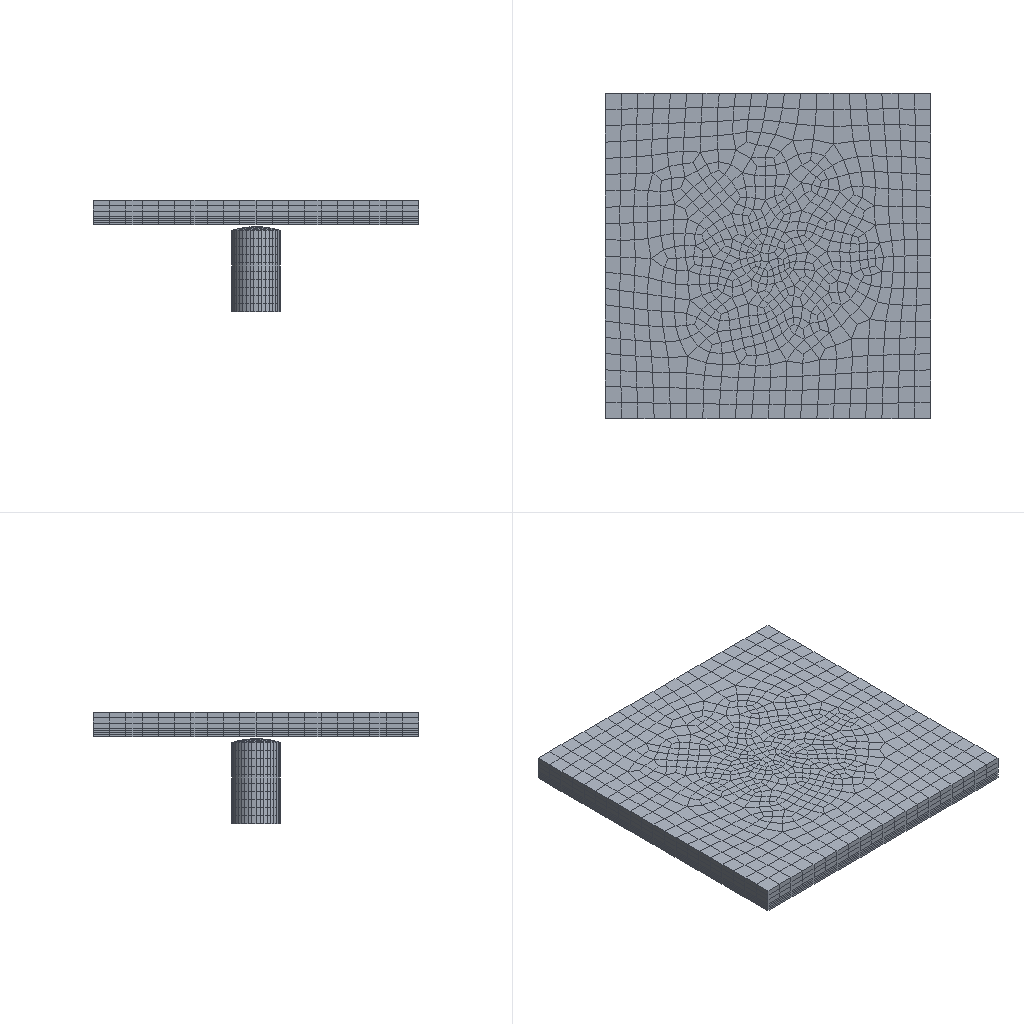Simulation study | abaqus
Set-up summary:
category,name,step,type,value,unit,region
solver,abaqus
solver,version,,,Abaqus/Explicit 2020
units,not stated in the deck,,not stated
analysis,deck,,transient,transient
load_step,Step-1,Step-1,transient
load_step,requested,,,1
mesh,nodes,,,12393
mesh,elements,,,7097
element_type,C3D8,,solid,7097
load,load commands in deck,,count,1
bc,support commands in deck,,count,7
material,GUODU,,in results
material,JIBAN,,in results
material,NAIMO,,in results
material,RIGID,,in results
check,setup vs results,,match,"per instance, exact: element labels, types and connectivity; labels of the nodes the elements use; coordinates not compared"
Abaqus input file, long lists of numbers shortened:
*Heading
** Job name: Job-2 Model name: Model-1
** Generated by: Abaqus/CAE 2020
*Preprint, echo=NO, model=NO, history=NO, contact=NO
**
** PARTS
**
*Part, name=guodu
*Node
      1,           0.,           0.,           0.
      2,         400.,           0.,           0.
** (2098 more lines like these left out)
*Element, type=C3D8
  1,  258,  227,  232,  262, 1089, 1058, 1063, 1093
  2,  981,  976,  472,  503, 1812, 1807, 1303, 1334
** (1007 more lines like these left out)
*Nset, nset=Set-1, generate
    1,  2100,     1
*Elset, elset=Set-1, generate
    1,  1009,     1
** Section: guodu
*Solid Section, elset=Set-1, material=guodu
,
*End Part
**
*Part, name=jiban
*Node
      1,           0.,           0.,           0.
      2,         400.,           0.,           0.
** (3030 more lines like these left out)
*Element, type=C3D8
   1,  106,  232,  756,  107, 1438, 1740, 2264, 1439
   2,   37,  280,  279,   38, 1607, 1788, 1787, 1606
** (2149 more lines like these left out)
*Nset, nset=Set-1, generate
    1,  3032,     1
*Elset, elset=Set-1, generate
    1,  2151,     1
** Section: jiban
*Solid Section, elset=Set-1, material=jiban
,
*End Part
**
*Part, name=naimo
*Node
      1,           0.,           0.,           0.
      2,         400.,           0.,           0.
** (1518 more lines like these left out)
*Element, type=C3D8
  1,   90,   89,  226,  240,  189,  188,  835,  849
  2,    5,  222,  740,   88,  186,  831, 1349,  187
** (717 more lines like these left out)
*Nset, nset=Set-1, generate
    1,  1520,     1
*Elset, elset=Set-1, generate
   1,  719,    1
** Section: naimo
*Solid Section, elset=Set-1, material=naimo
,
*End Part
**
*Part, name=rigid
*Node
      1,   20.173,   2.056,           0.
      2,   10.139,  0.5153,           0.
** (1538 more lines like these left out)
*Element, type=C3D8
   1,    1,    3,   81,  120,  141,  143,  221,  260
   2,    2,    1,   22,   24,  142,  141,  162,  164
** (1198 more lines like these left out)
*Node
   1541,           0.,   104.606, 1.83697009e-15
*Nset, nset=rigid-RefPt_, internal
1541,
*Nset, nset=Set-2, generate
    1,  1540,     1
*Elset, elset=Set-2, generate
    1,  1200,     1
** Section: rigid
*Solid Section, elset=Set-2, material=rigid
,
*End Part
**
**
** ASSEMBLY
**
*Assembly, name=Assembly
**
*Instance, name=guodu-1, part=guodu
*End Instance
**
*Instance, name=jiban-1, part=jiban
          0.,           0.,          2.5
*End Instance
**
*Instance, name=naimo-1, part=naimo
          0.,           0.,         -7.5
*End Instance
**
*Instance, name=guodu-2, part=guodu
          0.,           0.,         -2.5
*End Instance
**
*Instance, name=guodu-3, part=guodu
          0.,           0.,          -5.
*End Instance
**
*Instance, name=rigid-1, part=rigid
        200.,        -200.,         -10.
        200.,        -200.,         -10., 199.,        -200.,         -10., 90.
*End Instance
**
*Nset, nset=Set-1, instance=jiban-1
    7,    8,    9,   10,   11,  116,  117,  118,  119,  120,  121,  122,  123,  124,  125,  126
  127,  128,  129,  130,  131,  132,  133,  134,  135,  136,  137,  138,  139,  140,  141,  142
** (46 more lines like these left out)
*Elset, elset=Set-1, instance=jiban-1
 1327, 1328, 1329, 1330, 1331, 1332, 1333, 1334, 1335, 1336, 1337, 1338, 1339, 1340, 1341, 1342
 1343, 1344, 1345, 1346, 1347, 1348, 1349, 1350, 1351, 1352, 1353, 1354, 1355, 1356, 1357, 1358
** (43 more lines like these left out)
*Nset, nset=Set-2, instance=rigid-1
 1541,
*Nset, nset=Set-3, instance=rigid-1
    1,    2,    3,    4,    5,    6,    7,    8,    9,   10,   11,   12,   13,   14,   15,   16
   17,   18,   19,   20,   21,   22,   23,   24,   25,   26,   27,   28,   29,   30,   31,   32
** (37 more lines like these left out)
*Elset, elset=Set-3, instance=rigid-1
    1,    2,    3,    4,    5,    6,    7,    8,    9,   10,   11,   12,   13,   14,   15,   16
   17,   18,   19,   20,   21,   22,   23,   24,   25,   26,   27,   28,   29,   30,   31,   32
** (32 more lines like these left out)
*Nset, nset=Set-6, instance=rigid-1, generate
    1,  1540,     1
*Elset, elset=Set-6, instance=rigid-1, generate
    1,  1200,     1
*Nset, nset=Set-7, instance=rigid-1
 1541,
*Nset, nset=Set-8, instance=rigid-1
 1541,
*Nset, nset=Set-9, instance=rigid-1, generate
    1,  1541,     1
*Elset, elset=Set-9, instance=rigid-1, generate
    1,  1200,     1
*Nset, nset=Set-10, instance=rigid-1
 1541,
*Nset, nset=b_Set-4, instance=rigid-1, generate
    1,  1540,     1
*Elset, elset=b_Set-4, instance=rigid-1, generate
    1,  1200,     1
*Nset, nset=_PickedSet48, internal, instance=rigid-1
 1541,
*Elset, elset=_m_Surf-1_S1, internal, instance=jiban-1, generate
   1,  663,    1
*Surface, type=ELEMENT, name=m_Surf-1
_m_Surf-1_S1, S1
*Elset, elset=_m_Surf-3_S1, internal, instance=guodu-1, generate
   1,  887,    1
*Elset, elset=_m_Surf-3_S2, internal, instance=guodu-1, generate
  888,  1009,     1
*Surface, type=ELEMENT, name=m_Surf-3
_m_Surf-3_S1, S1
_m_Surf-3_S2, S2
*Elset, elset=_m_Surf-5_S1, internal, instance=guodu-2, generate
   1,  887,    1
*Elset, elset=_m_Surf-5_S2, internal, instance=guodu-2, generate
  888,  1009,     1
*Surface, type=ELEMENT, name=m_Surf-5
_m_Surf-5_S1, S1
_m_Surf-5_S2, S2
*Elset, elset=_m_Surf-7_S1, internal, instance=guodu-3, generate
   1,  887,    1
*Elset, elset=_m_Surf-7_S2, internal, instance=guodu-3, generate
  888,  1009,     1
*Surface, type=ELEMENT, name=m_Surf-7
_m_Surf-7_S1, S1
_m_Surf-7_S2, S2
*Elset, elset=_m_Surf-9_S4, internal, instance=rigid-1
    1,    6,   13,   16,   27,   39,   42,   43,   46,   58,   60,   81,   83,   84,   86,   89
   93,  105,  114,  115,  121,  126,  133,  136,  147,  159,  162,  163,  166,  178,  180,  201
** (11 more lines like these left out)
*Elset, elset=_m_Surf-9_S6, internal, instance=rigid-1
    7,   26,   37,   44,   47,   53,   54,   55,   56,   66,   74,   85,   88,   90,  127,  146
  157,  164,  167,  173,  174,  175,  176,  186,  194,  205,  208,  210,  247,  266,  277,  284
** (7 more lines like these left out)
*Elset, elset=_m_Surf-9_S3, internal, instance=rigid-1
   11,   59,  131,  179,  251,  299,  371,  419,  491,  539,  611,  659,  731,  779,  851,  899
  971, 1019, 1091, 1139
*Elset, elset=_m_Surf-9_S5, internal, instance=rigid-1
   12,   23,  132,  143,  252,  263,  372,  383,  492,  503,  612,  623,  732,  743,  852,  863
  972,  983, 1092, 1103
*Elset, elset=_m_Surf-9_S1, internal, instance=rigid-1, generate
   1,  120,    1
*Surface, type=ELEMENT, name=m_Surf-9
_m_Surf-9_S4, S4
_m_Surf-9_S6, S6
_m_Surf-9_S3, S3
_m_Surf-9_S5, S5
_m_Surf-9_S1, S1
*Elset, elset=_s_Surf-1_S2, internal, instance=guodu-1, generate
   1,  887,    1
*Elset, elset=_s_Surf-1_S1, internal, instance=guodu-1, generate
  888,  1009,     1
*Surface, type=ELEMENT, name=s_Surf-1
_s_Surf-1_S2, S2
_s_Surf-1_S1, S1
*Elset, elset=_s_Surf-3_S2, internal, instance=guodu-2, generate
   1,  887,    1
*Elset, elset=_s_Surf-3_S1, internal, instance=guodu-2, generate
  888,  1009,     1
*Surface, type=ELEMENT, name=s_Surf-3
_s_Surf-3_S2, S2
_s_Surf-3_S1, S1
*Elset, elset=_s_Surf-5_S2, internal, instance=guodu-3, generate
   1,  887,    1
*Elset, elset=_s_Surf-5_S1, internal, instance=guodu-3, generate
  888,  1009,     1
*Surface, type=ELEMENT, name=s_Surf-5
_s_Surf-5_S2, S2
_s_Surf-5_S1, S1
*Elset, elset=_s_Surf-7_S2, internal, instance=naimo-1, generate
   1,  660,    1
*Elset, elset=_s_Surf-7_S1, internal, instance=naimo-1, generate
 661,  719,    1
*Surface, type=ELEMENT, name=s_Surf-7
_s_Surf-7_S2, S2
_s_Surf-7_S1, S1
*Elset, elset=_s_Surf-9_S1, internal, instance=naimo-1, generate
   1,  660,    1
*Elset, elset=_s_Surf-9_S2, internal, instance=naimo-1, generate
 661,  719,    1
*Surface, type=ELEMENT, name=s_Surf-9
_s_Surf-9_S1, S1
_s_Surf-9_S2, S2
** Constraint: Constraint-1
*Tie, name=Constraint-1, adjust=yes
s_Surf-1, m_Surf-1
** Constraint: Constraint-2
*Tie, name=Constraint-2, adjust=yes
s_Surf-3, m_Surf-3
** Constraint: Constraint-3
*Tie, name=Constraint-3, adjust=yes
s_Surf-5, m_Surf-5
** Constraint: Constraint-4
*Tie, name=Constraint-4, adjust=yes
s_Surf-7, m_Surf-7
** Constraint: Constraint-5
*Rigid Body, ref node=_PickedSet48, elset=b_Set-4, position=CENTER OF MASS
*End Assembly
**
** MATERIALS
**
*Material, name=guodu
*Density
 7.74e-09,
*Elastic
206000., 0.29
*Plastic
420.,0.
*Material, name=jiban
*Density
 7.87e-09,
*Elastic
20700., 0.254
*Plastic
785.,0.
*Material, name=naimo
*Density
 7.86e-09,
*Elastic
212000., 0.289
*Plastic
835.,0.
*Material, name=rigid
*Density
 1.74e-08,
*Elastic
600000., 0.15
**
** INTERACTION PROPERTIES
**
*Surface Interaction, name=IntProp-1
*Friction
 0.3,
*Surface Behavior, pressure-overclosure=HARD
**
** INTERACTIONS
**
** Interaction: Int-2
*Contact, op=NEW
*Contact Inclusions, ALL EXTERIOR
*Contact Property Assignment
 ,  , IntProp-1
** ----------------------------------------------------------------
**
** STEP: Step-1
**
*Step, name=Step-1, nlgeom=YES
*Dynamic, Explicit
, 0.001
*Bulk Viscosity
0.06, 1.2
**
** BOUNDARY CONDITIONS
**
** Name: BC-1 Type: 对称/反对称/完全固定
*Boundary
Set-1, ENCASTRE
** Name: BC-3 Type: 速度/角速度
*Boundary, type=VELOCITY
Set-10, 1, 1
Set-10, 2, 2
Set-10, 3, 3, 11000.
Set-10, 4, 4
Set-10, 5, 5
Set-10, 6, 6
**
** INTERACTIONS
**
** Interaction: Int-1
*Contact Pair, interaction=IntProp-1, mechanical constraint=KINEMATIC, cpset=Int-1
m_Surf-9, s_Surf-9
**
** OUTPUT REQUESTS
**
*Restart, write, number interval=1, time marks=NO
**
** FIELD OUTPUT: F-Output-1
**
*Output, field, number interval=50
*Node Output
A, CF, RF, U, V
*Element Output, directions=YES
E, LE, MISES, PE, PEEQ, PEMAG, PS, S
*Contact Output
CDISP, CSTRESS
**
** HISTORY OUTPUT: H-Output-1
**
*Output, history, variable=PRESELECT, frequency=10
*End Step
Results summary:
result,step,Step-1,completed,increments=3271 time=0.001/0.001
result,analysis,,,transient
result,last_loadstep,,,1
result,primary field,,,U
result,reaction total,,FX,33216.96,model units
result,reaction total,,FY,-22294.616,model units
result,reaction total,,FZ,-648.292,model units